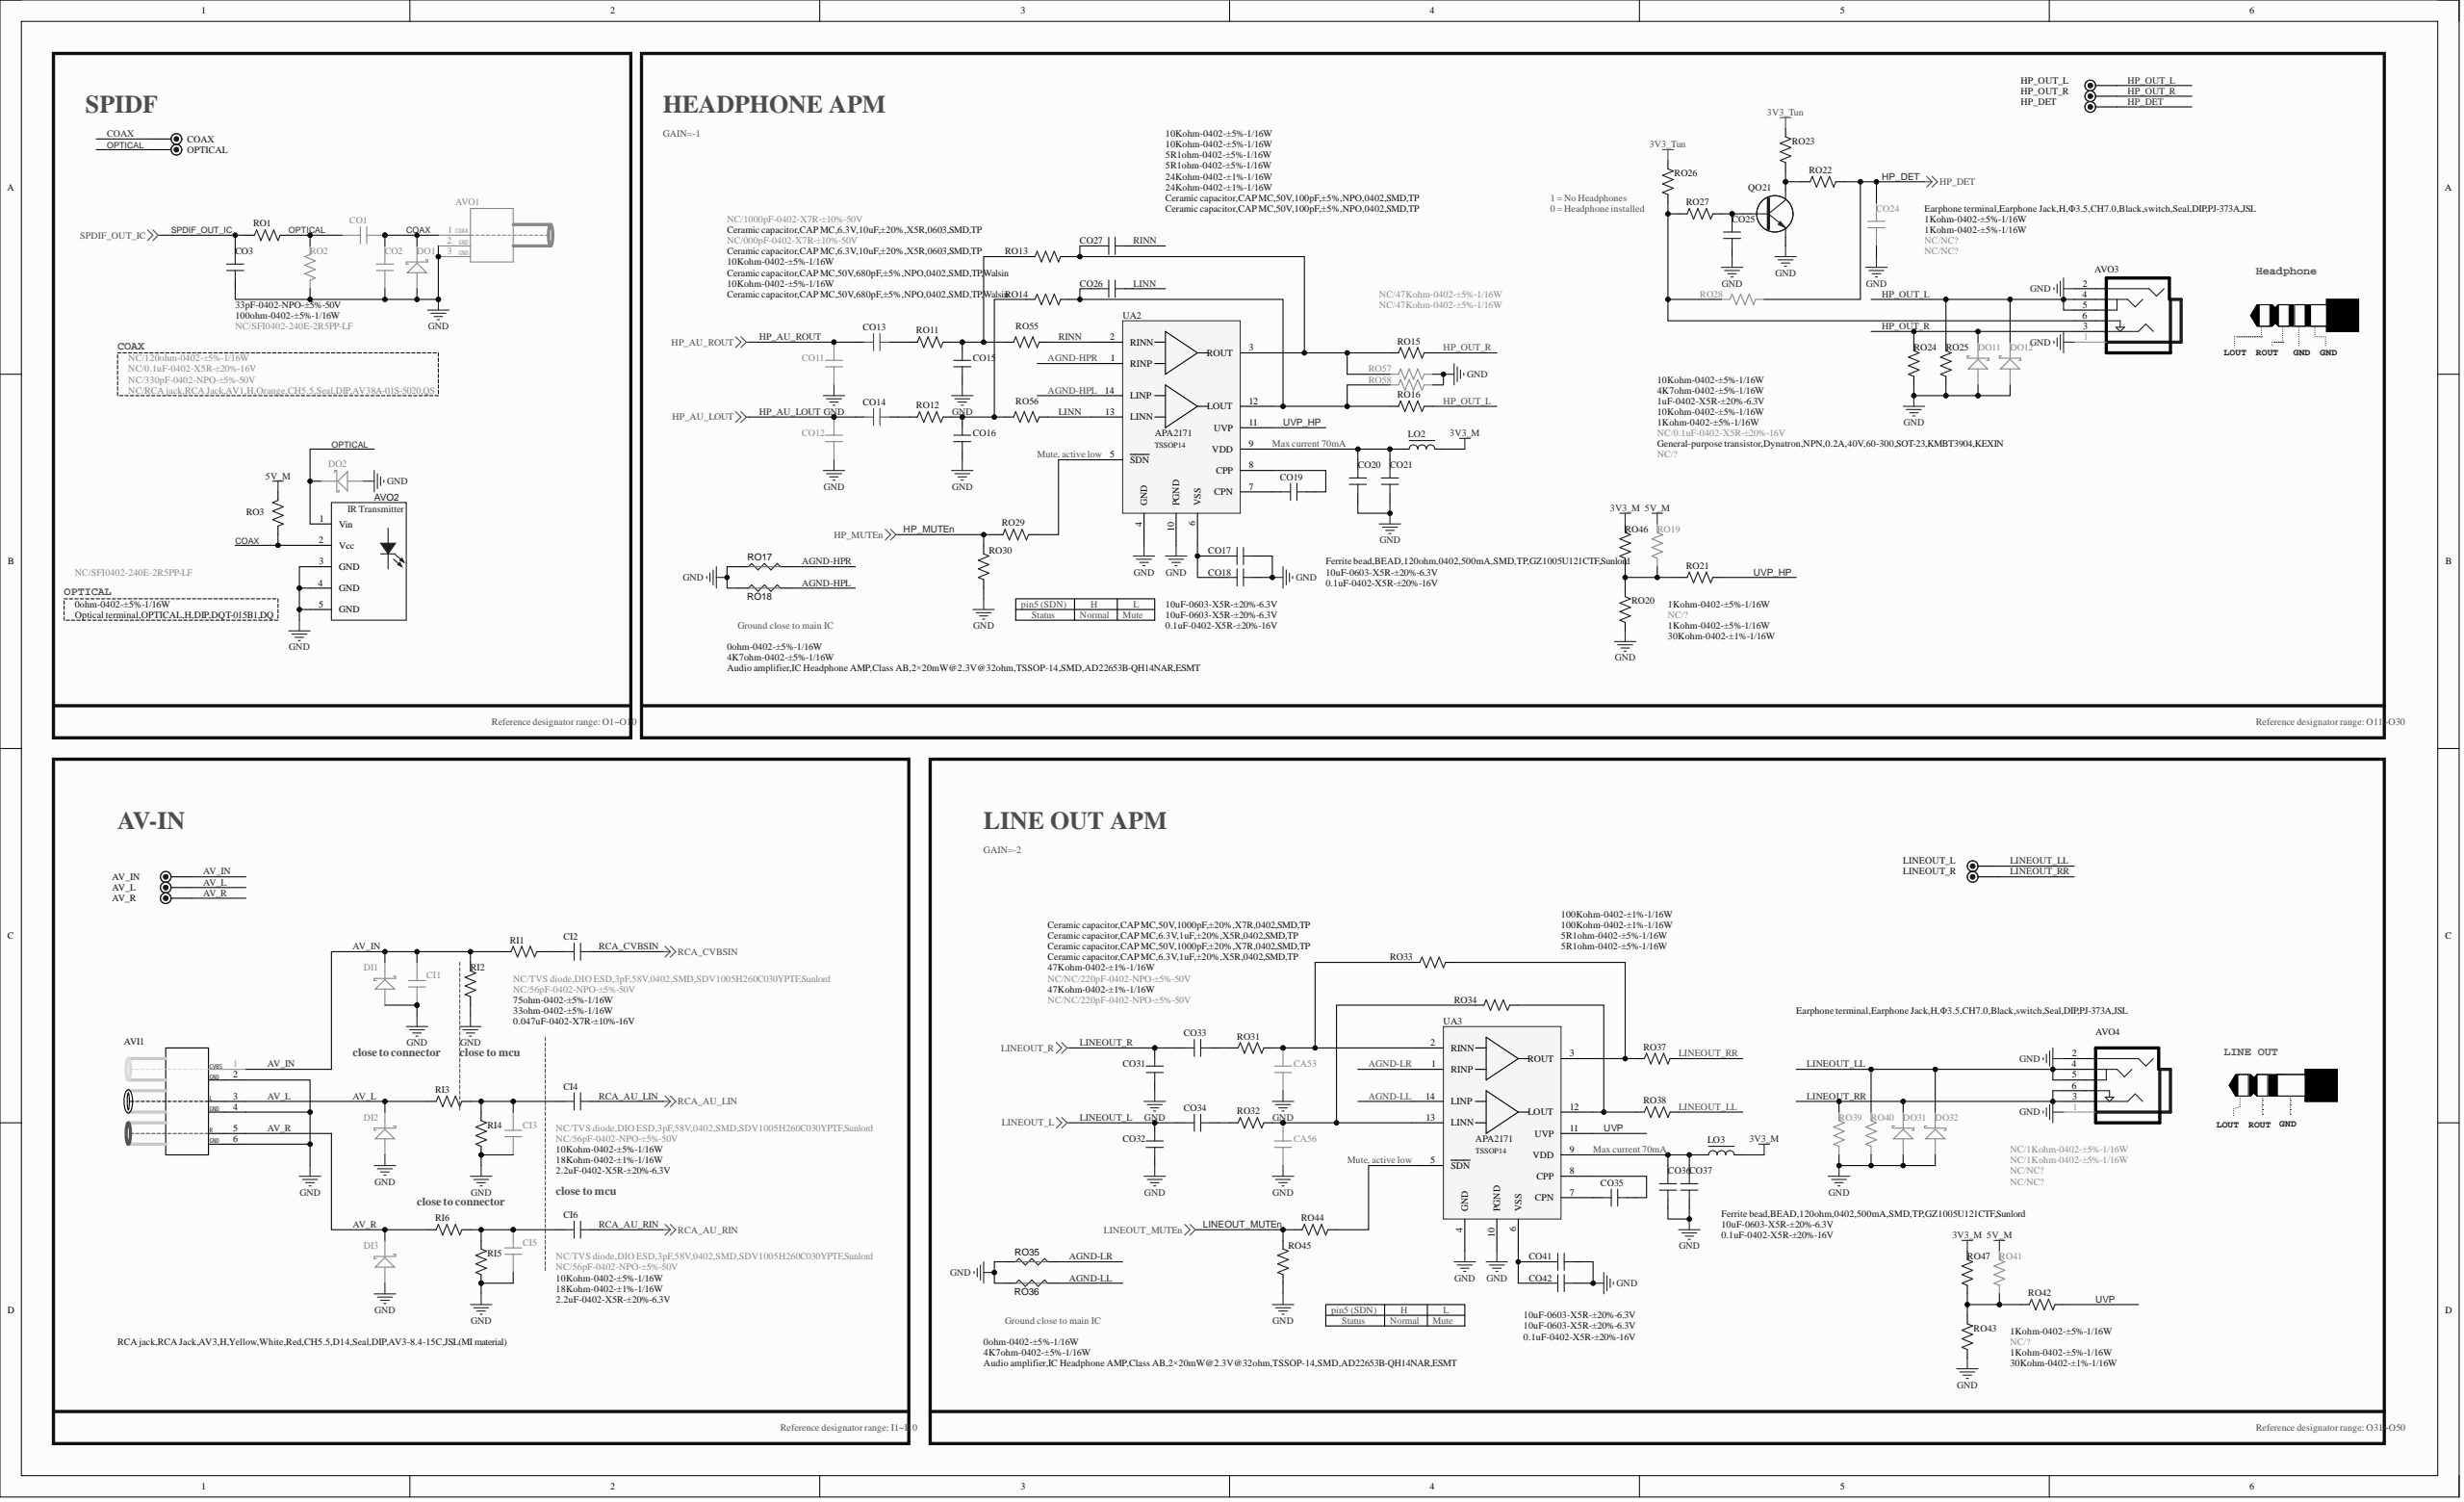Circuit board | Altium Designer | 1029 parts | 642 nets | one sheet of the schematic
Parts on this sheet (reference | value | footprint):
AV_IN | TEST | TP
AV_L | TEST | TP
AV_R | TEST | TP
AVI1 | RCA jack,RCA Jack,AV3,H,Yellow,White,Red,CH5.5,D14,Seal,DIP,AV3-8.4-15C,JSL(MI material) | AV3-H14-15
AVO1 | NC/RCA jack,RCA Jack,AV1,H,Orange,CH5.5,Seal,DIP,AV38A-01S-5020,QS | AV1-H-4
AVO2 | Optical terminal,OPTICAL,H,DIP,DQT-015B1,DQ | OPTICAL-HD-6
AVO3 | Earphone terminal,Earphone Jack,H,F3.5,CH7.0,Black,switch,Seal,DIP,PJ-373A,JSL | PHONE-HD-42
AVO4 | Earphone terminal,Earphone Jack,H,F3.5,CH7.0,Black,switch,Seal,DIP,PJ-373A,JSL | PHONE-HD-42
CA53 | NC/NC/220pF-0402-NPO-±5%-50V | C0402
CA56 | NC/NC/220pF-0402-NPO-±5%-50V | C0402
CI1 | NC/56pF-0402-NPO-±5%-50V | C0402
CI2 | 0.047uF-0402-X7R-±10%-16V | C0402
CI3 | NC/56pF-0402-NPO-±5%-50V | C0402
CI4 | 2.2uF-0402-X5R-±20%-6.3V | C0402
CI5 | NC/56pF-0402-NPO-±5%-50V | C0402
CI6 | 2.2uF-0402-X5R-±20%-6.3V | C0402
CO1 | NC/0.1uF-0402-X5R-±20%-16V | C0402
CO2 | NC/330pF-0402-NPO-±5%-50V | C0402
CO3 | 33pF-0402-NPO-±5%-50V | C0402
CO11 | NC/1000pF-0402-X7R-±10%-50V | C0402
CO12 | NC/000pF-0402-X7R-±10%-50V | C0402
CO13 | Ceramic capacitor,CAP MC,6.3V,10uF,±20%,X5R,0603,SMD,TP | C0603
CO14 | Ceramic capacitor,CAP MC,6.3V,10uF,±20%,X5R,0603,SMD,TP | C0603
CO15 | Ceramic capacitor,CAP MC,50V,680pF,±5%,NPO,0402,SMD,TP,Walsin | C0402
CO16 | Ceramic capacitor,CAP MC,50V,680pF,±5%,NPO,0402,SMD,TP,Walsin | C0402
CO17 | 10uF-0603-X5R-±20%-6.3V | C0603
CO18 | 0.1uF-0402-X5R-±20%-16V | C0402
CO19 | 10uF-0603-X5R-±20%-6.3V | C0603
CO20 | 10uF-0603-X5R-±20%-6.3V | C0603
CO21 | 0.1uF-0402-X5R-±20%-16V | C0402
CO24 | NC/0.1uF-0402-X5R-±20%-16V | C0402
CO25 | 1uF-0402-X5R-±20%-6.3V | C0402
CO26 | Ceramic capacitor,CAP MC,50V,100pF,±5%,NPO,0402,SMD,TP | C0402
CO27 | Ceramic capacitor,CAP MC,50V,100pF,±5%,NPO,0402,SMD,TP | C0402
CO31 | Ceramic capacitor,CAP MC,50V,1000pF,±20%,X7R,0402,SMD,TP | C0402
CO32 | Ceramic capacitor,CAP MC,50V,1000pF,±20%,X7R,0402,SMD,TP | C0402
CO33 | Ceramic capacitor,CAP MC,6.3V,1uF,±20%,X5R,0402,SMD,TP | C0402
CO34 | Ceramic capacitor,CAP MC,6.3V,1uF,±20%,X5R,0402,SMD,TP | C0402
CO35 | 10uF-0603-X5R-±20%-6.3V | C0603
CO36 | 10uF-0603-X5R-±20%-6.3V | C0603
CO37 | 0.1uF-0402-X5R-±20%-16V | C0402
CO41 | 10uF-0603-X5R-±20%-6.3V | C0603
CO42 | 0.1uF-0402-X5R-±20%-16V | C0402
COAX | TEST | TP
DI1 | NC/TVS diode,DIO ESD,3pF,58V,0402,SMD,SDV1005H260C030YPTF,Sunlord | DIODE-S0402
DI2 | NC/TVS diode,DIO ESD,3pF,58V,0402,SMD,SDV1005H260C030YPTF,Sunlord | DIODE-S0402
DI3 | NC/TVS diode,DIO ESD,3pF,58V,0402,SMD,SDV1005H260C030YPTF,Sunlord | DIODE-S0402
DO1 | NC/SFI0402-240E-2R5PP-LF | DIODE-S0402
DO2 | NC/SFI0402-240E-2R5PP-LF | DIODE-S0402
DO11 | NC/NC? | DIODE-S0402
DO12 | NC/NC? | DIODE-S0402
DO31 | NC/NC? | DIODE-S0402
DO32 | NC/NC? | DIODE-S0402
HP_OUT_L | TEST | TP
HP_OUT_R | TEST | TP
LINEOUT_L | TEST | TP
LINEOUT_R | TEST | TP
LO2 | Ferrite bead,BEAD,120ohm,0402,500mA,SMD,TP,GZ1005U121CTF,Sunlord | L0402
LO3 | Ferrite bead,BEAD,120ohm,0402,500mA,SMD,TP,GZ1005U121CTF,Sunlord | L0402
QO21 | General-purpose transistor,Dynatron,NPN,0.2A,40V,60-300,SOT-23,KMBT3904,KEXIN | SOT-23
RI1 | 33ohm-0402-±5%-1/16W | R0402
RI2 | 75ohm-0402-±5%-1/16W | R0402
RI3 | 10Kohm-0402-±5%-1/16W | R0402
RI4 | 18Kohm-0402-±1%-1/16W | R0402
RI5 | 18Kohm-0402-±1%-1/16W | R0402
RI6 | 10Kohm-0402-±5%-1/16W | R0402
RO1 | 100ohm-0402-±5%-1/16W | R0402
RO2 | NC/120ohm-0402-±5%-1/16W | R0402
RO3 | 0ohm-0402-±5%-1/16W | R0402
RO11 | 10Kohm-0402-±5%-1/16W | R0402
RO12 | 10Kohm-0402-±5%-1/16W | R0402
RO13 | 10Kohm-0402-±5%-1/16W | R0402
RO14 | 10Kohm-0402-±5%-1/16W | R0402
RO15 | 5R1ohm-0402-±5%-1/16W | R0402
RO16 | 5R1ohm-0402-±5%-1/16W | R0402
RO17 | NC/SHORT | GND
RO18 | NC/SHORT | GND
RO19 | NC/? | R0402
RO20 | 1Kohm-0402-±5%-1/16W | R0402
RO21 | 30Kohm-0402-±1%-1/16W | R0402
RO22 | 1Kohm-0402-±5%-1/16W | R0402
RO23 | 10Kohm-0402-±5%-1/16W | R0402
RO24 | 1Kohm-0402-±5%-1/16W | R0402
RO25 | 1Kohm-0402-±5%-1/16W | R0402
RO26 | 10Kohm-0402-±5%-1/16W | R0402
RO27 | 4K7ohm-0402-±5%-1/16W | R0402
RO28 | NC/? | R0402
RO29 | 0ohm-0402-±5%-1/16W | R0402
RO30 | 4K7ohm-0402-±5%-1/16W | R0402
RO31 | 47Kohm-0402-±1%-1/16W | R0402
RO32 | 47Kohm-0402-±1%-1/16W | R0402
RO33 | 100Kohm-0402-±1%-1/16W | R0402
RO34 | 100Kohm-0402-±1%-1/16W | R0402
RO35 | NC/SHORT | GND
RO36 | NC/SHORT | GND
RO37 | 5R1ohm-0402-±5%-1/16W | R0402
RO38 | 5R1ohm-0402-±5%-1/16W | R0402
RO39 | NC/1Kohm-0402-±5%-1/16W | R0402
RO40 | NC/1Kohm-0402-±5%-1/16W | R0402
RO41 | NC/? | R0402
RO42 | 30Kohm-0402-±1%-1/16W | R0402
RO43 | 1Kohm-0402-±5%-1/16W | R0402
RO44 | 0ohm-0402-±5%-1/16W | R0402
RO45 | 4K7ohm-0402-±5%-1/16W | R0402
RO46 | 1Kohm-0402-±5%-1/16W | R0402
RO47 | 1Kohm-0402-±5%-1/16W | R0402
RO55 | 24Kohm-0402-±1%-1/16W | R0402
RO56 | 24Kohm-0402-±1%-1/16W | R0402
RO57 | NC/47Kohm-0402-±5%-1/16W | R0402
RO58 | NC/47Kohm-0402-±5%-1/16W | R0402
UA2 | Audio amplifier,IC Headphone AMP,Class AB,2×20mW@2.3V@32ohm,TSSOP-14,SMD,AD22653B-QH14NAR,ESMT | SSOP14/0.65-1
UA3 | Audio amplifier,IC Headphone AMP,Class AB,2×20mW@2.3V@32ohm,TSSOP-14,SMD,AD22653B-QH14NAR,ESMT | SSOP14/0.65-1
Nets of these parts (net: part-pin ...):
UVP_HP: RO21-2 UA2-11
UVP: RO42-2 UA3-11
SPDIF_OUT_IC: CO3-2 RO1-1
RINN: CO27-2 RO55-2 UA2-2
RCA_CVBSIN: CI2-2
RCA_AU_RIN: CI6-2
RCA_AU_LIN: CI4-2
OPTICAL: AVO2-1 CO1-1 DO2-K RO1-2 RO2-2
NetRO44_2: RO44-2 UA3-5
NetRO41_1: RO41-1 RO42-1 RO43-2 RO47-1
NetRO34_2: RO34-2 RO38-1 UA3-12
NetRO33_2: RO33-2 RO37-1 UA3-3
NetRO29_2: RO29-2 UA2-5
NetRO19_1: RO19-1 RO20-2 RO21-1 RO46-1
NetQO21_C: QO21-C RO22-1 RO23-2
NetCO41_1: CO41-1 CO42-1 UA3-6
NetCO36_2: CO36-2 CO37-2 LO3-1 UA3-9
NetCO35_2: CO35-2 UA3-8
NetCO35_1: CO35-1 UA3-7
NetCO34_2: CO34-2 RO32-1
NetCO33_2: CO33-2 RO31-1
NetCO27_1: CO27-1 RO13-2 RO15-1 RO57-2 UA2-3
NetCO26_1: CO26-1 RO14-2 RO16-1 RO58-2 UA2-12
NetCO25_2: CO25-2 QO21-B RO27-1
NetCO20_2: CO20-2 CO21-2 LO2-1 UA2-9
NetCO19_2: CO19-2 UA2-8
NetCO19_1: CO19-1 UA2-7
NetCO17_1: CO17-1 CO18-1 UA2-6
NetCO16_2: CO16-2 RO12-2 RO14-1 RO56-1
NetCO15_2: CO15-2 RO11-2 RO13-1 RO55-1
NetCO14_1: CO14-1 RO12-1
NetCO13_1: CO13-1 RO11-1
NetCI5_2: CI5-2 CI6-1 RI5-2 RI6-2
NetCI3_2: CI3-2 CI4-1 RI3-2 RI4-2
NetCI2_1: CI2-1 RI1-2
NetCA56_2: CA56-2 RO32-2 RO34-1 UA3-13
NetCA53_2: CA53-2 RO31-2 RO33-1 UA3-2
NetAVO3_6: AVO3-6 RO26-2 RO27-2 RO28-1
LINN: CO26-2 RO56-2 UA2-13
LINEOUT_RR: AVO4-3 AVO4-6 DO31-K LINEOUT_R-1 RO37-2 RO39-2
LINEOUT_R: CO31-2 CO33-1
LINEOUT_MUTEn: RO44-1 RO45-2
LINEOUT_LL: AVO4-4 AVO4-5 DO32-K LINEOUT_L-1 RO38-2 RO40-2
LINEOUT_L: CO32-2 CO34-1
HP_OUT_R: AVO3-3 DO11-K HP_OUT_R-1 RO15-2 RO24-2
HP_OUT_L: AVO3-4 AVO3-5 DO12-K HP_OUT_L-1 RO16-2 RO25-2
HP_MUTEn: RO29-1 RO30-2
HP_DET: CO24-2 RO22-2 RO28-2
HP_AU_ROUT: CO11-2 CO13-2
HP_AU_LOUT: CO12-2 CO14-2
GND: AVI1-2 AVI1-4 AVI1-6 AVO1-2 AVO1-3 AVO2-3 AVO2-4 AVO2-5 AVO3-1 AVO3-2 AVO4-1 AVO4-2 CA53-1 CA56-1 CI1-1 CI3-1 CI5-1 CO2-1 CO3-1 CO11-1 CO12-1 CO15-1 CO16-1 CO17-2 CO18-2 CO20-1 CO21-1 CO24-1 CO25-1 CO31-1 CO32-1 CO36-1 CO37-1 CO41-2 CO42-2 DI1-A DI2-A DI3-A DO1-A DO2-A DO11-A DO12-A DO31-A DO32-A QO21-E RI2-1 RI4-1 RI5-1 RO2-1 RO17-JP_2K RO18-JP_2K RO20-1 RO24-1 RO25-1 RO30-1 RO35-JP_2K RO36-JP_2K RO39-1 RO40-1 RO43-1 RO45-1 RO57-1 RO58-1 UA2-4 UA2-10 UA3-4 UA3-10
COAX: AVO1-1 AVO2-2 CO1-2 CO2-2 COAX-1 DO1-K RO3-2
AV_R: AVI1-5 AV_R-1 DI3-K RI6-1
AV_L: AVI1-3 AV_L-1 DI2-K RI3-1
AV_IN: AVI1-1 AV_IN-1 CI1-2 DI1-K RI1-1 RI2-2
AGND-LR: RO35-JP_1K UA3-1
AGND-LL: RO36-JP_1K UA3-14
AGND-HPR: RO17-JP_1K UA2-1
AGND-HPL: RO18-JP_1K UA2-14
5V_M: RO3-1 RO19-2 RO41-2
3V3_Tun: RO23-1 RO26-1
3V3_M: LO2-2 LO3-2 RO46-2 RO47-2